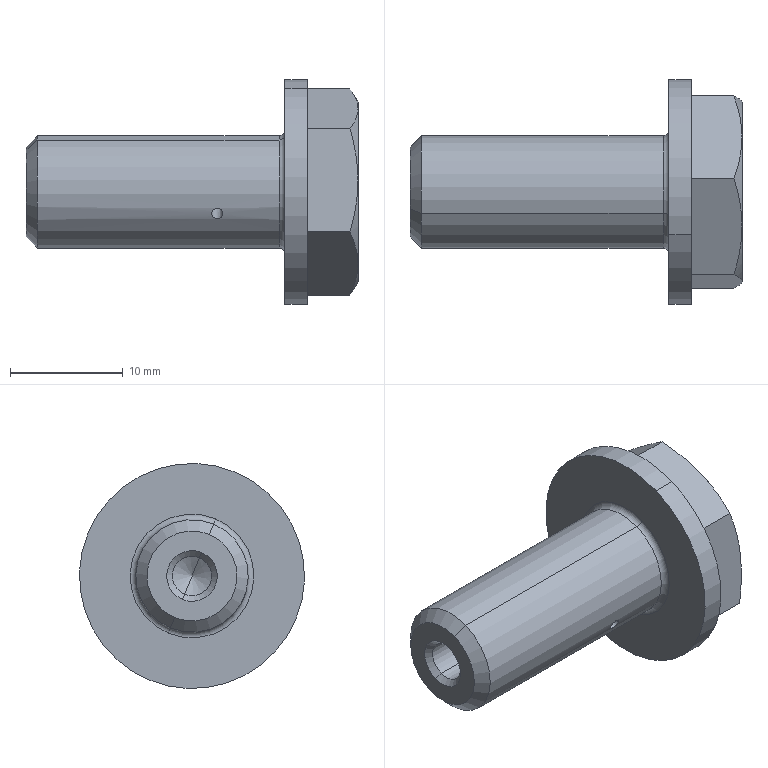Part | SolidWorks | features BaseBody 1 | 1 solid | 32 faces | box 29.5 x 20 x 20 mm | volume 3225 mm3 | cone 12 | plane 10 | cylinder 8 | torus 2 | commonest cylinder face diameters 1 x2 3.5 x2 10 x2 20 x2
STEP:
#1=CARTESIAN_POINT('',(464.9,22.643,5.081));
#2=VERTEX_POINT('',#1);
#3=CARTESIAN_POINT('',(464.9,26.857,-5.081));
#4=VERTEX_POINT('',#3);
#5=CARTESIAN_POINT('',(464.9,24.75,0.));
#6=DIRECTION('',(1.,0.,0.));
#7=DIRECTION('',(0.,0.383,-0.9237));
#8=AXIS2_PLACEMENT_3D('',#5,#6,#7);
#9=CIRCLE('',#8,5.5);
#10=EDGE_CURVE('',#2,#4,#9,.T.);
#11=ORIENTED_EDGE('',*,*,#10,.F.);
#12=CARTESIAN_POINT('',(464.4,22.835,4.619));
#13=VERTEX_POINT('',#12);
#14=CARTESIAN_POINT('',(464.4,22.643,5.081));
#15=DIRECTION('',(0.,0.9237,0.383));
#16=DIRECTION('',(0.,-0.383,0.9237));
#17=AXIS2_PLACEMENT_3D('',#14,#15,#16);
#18=CIRCLE('',#17,0.5);
#19=EDGE_CURVE('',#2,#13,#18,.T.);
#20=ORIENTED_EDGE('',*,*,#19,.T.);
#21=CARTESIAN_POINT('',(464.4,26.665,-4.619));
#22=VERTEX_POINT('',#21);
#23=CARTESIAN_POINT('',(464.4,24.75,0.));
#24=DIRECTION('',(-1.,0.,0.));
#25=DIRECTION('',(0.,0.383,-0.9237));
#26=AXIS2_PLACEMENT_3D('',#23,#24,#25);
#27=CIRCLE('',#26,5.);
#28=EDGE_CURVE('',#22,#13,#27,.T.);
#29=ORIENTED_EDGE('',*,*,#28,.F.);
#30=CARTESIAN_POINT('',(464.4,26.857,-5.081));
#31=DIRECTION('',(0.,-0.9237,-0.383));
#32=DIRECTION('',(0.,0.383,-0.9237));
#33=AXIS2_PLACEMENT_3D('',#30,#31,#32);
#34=CIRCLE('',#33,0.5);
#35=EDGE_CURVE('',#4,#22,#34,.T.);
#36=ORIENTED_EDGE('',*,*,#35,.F.);
#37=EDGE_LOOP('',(#11,#20,#29,#36));
#38=FACE_OUTER_BOUND('',#37,.T.);
#39=CARTESIAN_POINT('',(464.4,24.75,0.));
#40=DIRECTION('',(1.,0.,0.));
#41=DIRECTION('',(0.,0.383,-0.9237));
#42=AXIS2_PLACEMENT_3D('',#39,#40,#41);
#43=TOROIDAL_SURFACE('',#42,5.5,0.5);
#44=ADVANCED_FACE('',(#38),#43,.F.);
#45=CARTESIAN_POINT('',(442.4,25.42,-1.617));
#46=VERTEX_POINT('',#45);
#47=CARTESIAN_POINT('',(442.4,24.08,1.617));
#48=VERTEX_POINT('',#47);
#49=CARTESIAN_POINT('',(442.4,24.75,0.));
#50=DIRECTION('',(-1.,0.,0.));
#51=DIRECTION('',(0.,-0.383,0.9237));
#52=AXIS2_PLACEMENT_3D('',#49,#50,#51);
#53=CIRCLE('',#52,1.75);
#54=EDGE_CURVE('',#46,#48,#53,.T.);
#55=ORIENTED_EDGE('',*,*,#54,.F.);
#56=CARTESIAN_POINT('',(441.9,25.612,-2.078));
#57=VERTEX_POINT('',#56);
#58=CARTESIAN_POINT('',(442.4,25.42,-1.617));
#59=DIRECTION('',(-0.7071,0.2709,-0.6532));
#60=VECTOR('',#59,1000.);
#61=LINE('',#58,#60);
#62=EDGE_CURVE('',#46,#57,#61,.T.);
#63=ORIENTED_EDGE('',*,*,#62,.T.);
#64=CARTESIAN_POINT('',(441.9,23.888,2.078));
#65=VERTEX_POINT('',#64);
#66=CARTESIAN_POINT('',(441.9,24.75,0.));
#67=DIRECTION('',(1.,0.,0.));
#68=DIRECTION('',(0.,-0.383,0.9237));
#69=AXIS2_PLACEMENT_3D('',#66,#67,#68);
#70=CIRCLE('',#69,2.25);
#71=EDGE_CURVE('',#65,#57,#70,.T.);
#72=ORIENTED_EDGE('',*,*,#71,.F.);
#73=CARTESIAN_POINT('',(442.4,24.08,1.617));
#74=DIRECTION('',(-0.7071,-0.2709,0.6532));
#75=VECTOR('',#74,1000.);
#76=LINE('',#73,#75);
#77=EDGE_CURVE('',#48,#65,#76,.T.);
#78=ORIENTED_EDGE('',*,*,#77,.F.);
#79=EDGE_LOOP('',(#55,#63,#72,#78));
#80=FACE_OUTER_BOUND('',#79,.T.);
#81=CARTESIAN_POINT('',(442.4,24.75,0.));
#82=DIRECTION('',(-1.,0.,0.));
#83=DIRECTION('',(0.,-0.383,0.9237));
#84=AXIS2_PLACEMENT_3D('',#81,#82,#83);
#85=CONICAL_SURFACE('',#84,1.75,0.7854);
#86=ADVANCED_FACE('',(#80),#85,.F.);
#87=CARTESIAN_POINT('',(461.91,24.75,0.));
#88=VERTEX_POINT('',#87);
#89=CARTESIAN_POINT('',(460.9,24.08,1.617));
#90=VERTEX_POINT('',#89);
#91=CARTESIAN_POINT('',(460.9,24.08,1.617));
#92=DIRECTION('',(-0.5,-0.3317,0.8));
#93=VECTOR('',#92,1000.);
#94=LINE('',#91,#93);
#95=EDGE_CURVE('',#88,#90,#94,.T.);
#96=ORIENTED_EDGE('',*,*,#95,.F.);
#97=CARTESIAN_POINT('',(460.9,25.42,-1.617));
#98=VERTEX_POINT('',#97);
#99=CARTESIAN_POINT('',(460.9,25.42,-1.617));
#100=DIRECTION('',(-0.5,0.3317,-0.8));
#101=VECTOR('',#100,1000.);
#102=LINE('',#99,#101);
#103=EDGE_CURVE('',#88,#98,#102,.T.);
#104=ORIENTED_EDGE('',*,*,#103,.T.);
#105=CARTESIAN_POINT('',(460.9,24.75,0.));
#106=DIRECTION('',(-1.,0.,0.));
#107=DIRECTION('',(0.,-0.383,0.9237));
#108=AXIS2_PLACEMENT_3D('',#105,#106,#107);
#109=CIRCLE('',#108,1.75);
#110=EDGE_CURVE('',#98,#90,#109,.T.);
#111=ORIENTED_EDGE('',*,*,#110,.T.);
#112=EDGE_LOOP('',(#96,#104,#111));
#113=FACE_OUTER_BOUND('',#112,.T.);
#114=CARTESIAN_POINT('',(460.9,24.75,0.));
#115=DIRECTION('',(-1.,0.,0.));
#116=DIRECTION('',(0.,-0.383,0.9237));
#117=AXIS2_PLACEMENT_3D('',#114,#115,#116);
#118=CONICAL_SURFACE('',#117,1.75,1.047);
#119=ADVANCED_FACE('',(#113),#118,.F.);
#120=CARTESIAN_POINT('',(458.4,23.133,-0.6703));
#121=VERTEX_POINT('',#120);
#122=CARTESIAN_POINT('',(459.4,23.133,-0.6703));
#123=VERTEX_POINT('',#122);
#124=CARTESIAN_POINT('',(458.4,23.133,-0.6703));
#125=CARTESIAN_POINT('',(458.4,23.083,-0.5476));
#126=CARTESIAN_POINT('',(458.455,23.049,-0.4218));
#127=CARTESIAN_POINT('',(458.638,23.014,-0.2378));
#128=CARTESIAN_POINT('',(458.769,23.009,-0.1806));
#129=CARTESIAN_POINT('',(459.031,23.009,-0.1805));
#130=CARTESIAN_POINT('',(459.161,23.014,-0.2374));
#131=CARTESIAN_POINT('',(459.346,23.049,-0.4227));
#132=CARTESIAN_POINT('',(459.4,23.083,-0.5494));
#133=CARTESIAN_POINT('',(459.4,23.133,-0.6703));
#134=B_SPLINE_CURVE_WITH_KNOTS('',3,(#124,#125,#126,#127,#128,#129,#130,#131,#132,#133),.UNSPECIFIED.,.F.,.F.,(4,2,2,2,4),(0.,0.0003929,0.0007857,0.001179,0.001571),.UNSPECIFIED.);
#135=EDGE_CURVE('',#121,#123,#134,.T.);
#136=ORIENTED_EDGE('',*,*,#135,.F.);
#137=CARTESIAN_POINT('',(459.4,23.133,-0.6703));
#138=CARTESIAN_POINT('',(459.4,23.184,-0.7913));
#139=CARTESIAN_POINT('',(459.346,23.249,-0.9051));
#140=CARTESIAN_POINT('',(459.161,23.355,-1.061));
#141=CARTESIAN_POINT('',(459.032,23.392,-1.104));
#142=CARTESIAN_POINT('',(458.768,23.392,-1.104));
#143=CARTESIAN_POINT('',(458.638,23.355,-1.061));
#144=CARTESIAN_POINT('',(458.455,23.25,-0.9058));
#145=CARTESIAN_POINT('',(458.4,23.184,-0.7931));
#146=CARTESIAN_POINT('',(458.4,23.133,-0.6703));
#147=B_SPLINE_CURVE_WITH_KNOTS('',3,(#137,#138,#139,#140,#141,#142,#143,#144,#145,#146),.UNSPECIFIED.,.F.,.F.,(4,2,2,2,4),(0.001571,0.001964,0.002357,0.00275,0.003142),.UNSPECIFIED.);
#148=EDGE_CURVE('',#123,#121,#147,.T.);
#149=ORIENTED_EDGE('',*,*,#148,.F.);
#150=EDGE_LOOP('',(#136,#149));
#151=FACE_BOUND('',#150,.T.);
#152=ORIENTED_EDGE('',*,*,#110,.F.);
#153=CARTESIAN_POINT('',(441.9,25.42,-1.617));
#154=DIRECTION('',(-1.,0.,0.));
#155=VECTOR('',#154,1000.);
#156=LINE('',#153,#155);
#157=EDGE_CURVE('',#98,#46,#156,.T.);
#158=ORIENTED_EDGE('',*,*,#157,.T.);
#159=ORIENTED_EDGE('',*,*,#54,.T.);
#160=CARTESIAN_POINT('',(441.9,24.08,1.617));
#161=DIRECTION('',(-1.,0.,0.));
#162=VECTOR('',#161,1000.);
#163=LINE('',#160,#162);
#164=EDGE_CURVE('',#90,#48,#163,.T.);
#165=ORIENTED_EDGE('',*,*,#164,.F.);
#166=EDGE_LOOP('',(#152,#158,#159,#165));
#167=FACE_OUTER_BOUND('',#166,.T.);
#168=CARTESIAN_POINT('',(441.9,24.75,0.));
#169=DIRECTION('',(-1.,0.,0.));
#170=DIRECTION('',(0.,-0.383,0.9237));
#171=AXIS2_PLACEMENT_3D('',#168,#169,#170);
#172=CYLINDRICAL_SURFACE('',#171,1.75);
#173=ADVANCED_FACE('',(#151,#167),#172,.F.);
#174=CARTESIAN_POINT('',(466.9,20.92,9.237));
#175=VERTEX_POINT('',#174);
#176=CARTESIAN_POINT('',(466.9,28.58,-9.237));
#177=VERTEX_POINT('',#176);
#178=CARTESIAN_POINT('',(466.9,24.75,0.));
#179=DIRECTION('',(-1.,0.,0.));
#180=DIRECTION('',(0.,-0.383,0.9237));
#181=AXIS2_PLACEMENT_3D('',#178,#179,#180);
#182=CIRCLE('',#181,10.);
#183=EDGE_CURVE('',#175,#177,#182,.T.);
#184=ORIENTED_EDGE('',*,*,#183,.T.);
#185=CARTESIAN_POINT('',(464.9,28.58,-9.237));
#186=VERTEX_POINT('',#185);
#187=CARTESIAN_POINT('',(466.9,28.58,-9.237));
#188=DIRECTION('',(-1.,0.,0.));
#189=VECTOR('',#188,1000.);
#190=LINE('',#187,#189);
#191=EDGE_CURVE('',#177,#186,#190,.T.);
#192=ORIENTED_EDGE('',*,*,#191,.T.);
#193=CARTESIAN_POINT('',(464.9,20.92,9.237));
#194=VERTEX_POINT('',#193);
#195=CARTESIAN_POINT('',(464.9,24.75,0.));
#196=DIRECTION('',(-1.,0.,0.));
#197=DIRECTION('',(0.,-0.383,0.9237));
#198=AXIS2_PLACEMENT_3D('',#195,#196,#197);
#199=CIRCLE('',#198,10.);
#200=EDGE_CURVE('',#194,#186,#199,.T.);
#201=ORIENTED_EDGE('',*,*,#200,.F.);
#202=CARTESIAN_POINT('',(466.9,20.92,9.237));
#203=DIRECTION('',(-1.,0.,0.));
#204=VECTOR('',#203,1000.);
#205=LINE('',#202,#204);
#206=EDGE_CURVE('',#175,#194,#205,.T.);
#207=ORIENTED_EDGE('',*,*,#206,.F.);
#208=EDGE_LOOP('',(#184,#192,#201,#207));
#209=FACE_OUTER_BOUND('',#208,.T.);
#210=CARTESIAN_POINT('',(466.9,24.75,0.));
#211=DIRECTION('',(-1.,0.,0.));
#212=DIRECTION('',(0.,-0.383,0.9237));
#213=AXIS2_PLACEMENT_3D('',#210,#211,#212);
#214=CYLINDRICAL_SURFACE('',#213,10.);
#215=ADVANCED_FACE('',(#209),#214,.T.);
#216=CARTESIAN_POINT('',(459.4,20.131,-1.915));
#217=VERTEX_POINT('',#216);
#218=CARTESIAN_POINT('',(458.4,20.131,-1.915));
#219=VERTEX_POINT('',#218);
#220=CARTESIAN_POINT('',(459.4,20.131,-1.915));
#221=CARTESIAN_POINT('',(459.4,20.181,-2.036));
#222=CARTESIAN_POINT('',(459.346,20.237,-2.154));
#223=CARTESIAN_POINT('',(459.162,20.32,-2.32));
#224=CARTESIAN_POINT('',(459.033,20.346,-2.367));
#225=CARTESIAN_POINT('',(458.768,20.346,-2.368));
#226=CARTESIAN_POINT('',(458.639,20.32,-2.32));
#227=CARTESIAN_POINT('',(458.454,20.237,-2.155));
#228=CARTESIAN_POINT('',(458.4,20.182,-2.037));
#229=CARTESIAN_POINT('',(458.4,20.131,-1.915));
#230=B_SPLINE_CURVE_WITH_KNOTS('',3,(#220,#221,#222,#223,#224,#225,#226,#227,#228,#229),.UNSPECIFIED.,.F.,.F.,(4,2,2,2,4),(0.001564,0.001955,0.002346,0.002737,0.003128),.UNSPECIFIED.);
#231=EDGE_CURVE('',#217,#219,#230,.T.);
#232=ORIENTED_EDGE('',*,*,#231,.F.);
#233=CARTESIAN_POINT('',(459.4,16.217,-3.538));
#234=DIRECTION('',(0.,0.9237,0.383));
#235=VECTOR('',#234,1000.);
#236=LINE('',#233,#235);
#237=EDGE_CURVE('',#217,#123,#236,.T.);
#238=ORIENTED_EDGE('',*,*,#237,.T.);
#239=ORIENTED_EDGE('',*,*,#148,.T.);
#240=CARTESIAN_POINT('',(458.4,16.217,-3.538));
#241=DIRECTION('',(0.,0.9237,0.383));
#242=VECTOR('',#241,1000.);
#243=LINE('',#240,#242);
#244=EDGE_CURVE('',#219,#121,#243,.T.);
#245=ORIENTED_EDGE('',*,*,#244,.F.);
#246=EDGE_LOOP('',(#232,#238,#239,#245));
#247=FACE_OUTER_BOUND('',#246,.T.);
#248=CARTESIAN_POINT('',(458.9,16.217,-3.538));
#249=DIRECTION('',(0.,0.9237,0.383));
#250=DIRECTION('',(-1.,0.,0.));
#251=AXIS2_PLACEMENT_3D('',#248,#249,#250);
#252=CYLINDRICAL_SURFACE('',#251,0.5);
#253=ADVANCED_FACE('',(#247),#252,.F.);
#254=CARTESIAN_POINT('',(441.9,23.218,3.695));
#255=VERTEX_POINT('',#254);
#256=CARTESIAN_POINT('',(441.9,26.282,-3.695));
#257=VERTEX_POINT('',#256);
#258=CARTESIAN_POINT('',(441.9,24.75,0.));
#259=DIRECTION('',(-1.,0.,0.));
#260=DIRECTION('',(0.,-0.383,0.9237));
#261=AXIS2_PLACEMENT_3D('',#258,#259,#260);
#262=CIRCLE('',#261,4.);
#263=EDGE_CURVE('',#255,#257,#262,.T.);
#264=ORIENTED_EDGE('',*,*,#263,.F.);
#265=CARTESIAN_POINT('',(442.9,22.835,4.619));
#266=VERTEX_POINT('',#265);
#267=CARTESIAN_POINT('',(441.9,23.218,3.695));
#268=DIRECTION('',(0.7071,-0.2709,0.6532));
#269=VECTOR('',#268,1000.);
#270=LINE('',#267,#269);
#271=EDGE_CURVE('',#255,#266,#270,.T.);
#272=ORIENTED_EDGE('',*,*,#271,.T.);
#273=CARTESIAN_POINT('',(442.9,26.665,-4.619));
#274=VERTEX_POINT('',#273);
#275=CARTESIAN_POINT('',(442.9,24.75,0.));
#276=DIRECTION('',(1.,0.,0.));
#277=DIRECTION('',(0.,-0.383,0.9237));
#278=AXIS2_PLACEMENT_3D('',#275,#276,#277);
#279=CIRCLE('',#278,5.);
#280=EDGE_CURVE('',#274,#266,#279,.T.);
#281=ORIENTED_EDGE('',*,*,#280,.F.);
#282=CARTESIAN_POINT('',(441.9,26.282,-3.695));
#283=DIRECTION('',(0.7071,0.2709,-0.6532));
#284=VECTOR('',#283,1000.);
#285=LINE('',#282,#284);
#286=EDGE_CURVE('',#257,#274,#285,.T.);
#287=ORIENTED_EDGE('',*,*,#286,.F.);
#288=EDGE_LOOP('',(#264,#272,#281,#287));
#289=FACE_OUTER_BOUND('',#288,.T.);
#290=CARTESIAN_POINT('',(441.9,24.75,0.));
#291=DIRECTION('',(1.,0.,0.));
#292=DIRECTION('',(0.,0.383,-0.9237));
#293=AXIS2_PLACEMENT_3D('',#290,#291,#292);
#294=CONICAL_SURFACE('',#293,4.,0.7854);
#295=ADVANCED_FACE('',(#289),#294,.T.);
#296=ORIENTED_EDGE('',*,*,#280,.T.);
#297=CARTESIAN_POINT('',(441.9,22.835,4.619));
#298=DIRECTION('',(1.,0.,0.));
#299=VECTOR('',#298,1000.);
#300=LINE('',#297,#299);
#301=EDGE_CURVE('',#266,#13,#300,.T.);
#302=ORIENTED_EDGE('',*,*,#301,.T.);
#303=CARTESIAN_POINT('',(464.4,24.75,0.));
#304=DIRECTION('',(-1.,0.,0.));
#305=DIRECTION('',(0.,0.383,-0.9237));
#306=AXIS2_PLACEMENT_3D('',#303,#304,#305);
#307=CIRCLE('',#306,5.);
#308=EDGE_CURVE('',#13,#22,#307,.T.);
#309=ORIENTED_EDGE('',*,*,#308,.T.);
#310=CARTESIAN_POINT('',(441.9,26.665,-4.619));
#311=DIRECTION('',(1.,0.,0.));
#312=VECTOR('',#311,1000.);
#313=LINE('',#310,#312);
#314=EDGE_CURVE('',#274,#22,#313,.T.);
#315=ORIENTED_EDGE('',*,*,#314,.F.);
#316=EDGE_LOOP('',(#296,#302,#309,#315));
#317=FACE_OUTER_BOUND('',#316,.T.);
#318=CARTESIAN_POINT('',(441.9,24.75,0.));
#319=DIRECTION('',(1.,0.,0.));
#320=DIRECTION('',(0.,0.383,-0.9237));
#321=AXIS2_PLACEMENT_3D('',#318,#319,#320);
#322=CYLINDRICAL_SURFACE('',#321,5.);
#323=ADVANCED_FACE('',(#317),#322,.T.);
#324=CARTESIAN_POINT('',(464.9,24.75,0.));
#325=DIRECTION('',(1.,0.,0.));
#326=DIRECTION('',(0.,0.383,-0.9237));
#327=AXIS2_PLACEMENT_3D('',#324,#325,#326);
#328=CIRCLE('',#327,5.5);
#329=EDGE_CURVE('',#4,#2,#328,.T.);
#330=ORIENTED_EDGE('',*,*,#329,.T.);
#331=ORIENTED_EDGE('',*,*,#10,.T.);
#332=EDGE_LOOP('',(#330,#331));
#333=FACE_BOUND('',#332,.T.);
#334=ORIENTED_EDGE('',*,*,#200,.T.);
#335=CARTESIAN_POINT('',(464.9,24.75,0.));
#336=DIRECTION('',(-1.,0.,0.));
#337=DIRECTION('',(0.,-0.383,0.9237));
#338=AXIS2_PLACEMENT_3D('',#335,#336,#337);
#339=CIRCLE('',#338,10.);
#340=EDGE_CURVE('',#186,#194,#339,.T.);
#341=ORIENTED_EDGE('',*,*,#340,.T.);
#342=EDGE_LOOP('',(#334,#341));
#343=FACE_OUTER_BOUND('',#342,.T.);
#344=CARTESIAN_POINT('',(464.9,30.879,-14.78));
#345=DIRECTION('',(1.,0.,0.));
#346=DIRECTION('',(0.,0.383,-0.9237));
#347=AXIS2_PLACEMENT_3D('',#344,#345,#346);
#348=PLANE('',#347);
#349=ADVANCED_FACE('',(#333,#343),#348,.F.);
#350=ORIENTED_EDGE('',*,*,#301,.F.);
#351=CARTESIAN_POINT('',(442.9,24.75,0.));
#352=DIRECTION('',(1.,0.,0.));
#353=DIRECTION('',(0.,-0.383,0.9237));
#354=AXIS2_PLACEMENT_3D('',#351,#352,#353);
#355=CIRCLE('',#354,5.);
#356=EDGE_CURVE('',#266,#274,#355,.T.);
#357=ORIENTED_EDGE('',*,*,#356,.T.);
#358=ORIENTED_EDGE('',*,*,#314,.T.);
#359=ORIENTED_EDGE('',*,*,#28,.T.);
#360=EDGE_LOOP('',(#350,#357,#358,#359));
#361=FACE_OUTER_BOUND('',#360,.T.);
#362=CARTESIAN_POINT('',(458.4,20.131,-1.915));
#363=CARTESIAN_POINT('',(458.4,20.081,-1.793));
#364=CARTESIAN_POINT('',(458.454,20.037,-1.671));
#365=CARTESIAN_POINT('',(458.639,19.978,-1.496));
#366=CARTESIAN_POINT('',(458.769,19.963,-1.444));
#367=CARTESIAN_POINT('',(459.03,19.963,-1.444));
#368=CARTESIAN_POINT('',(459.16,19.978,-1.495));
#369=CARTESIAN_POINT('',(459.347,20.037,-1.673));
#370=CARTESIAN_POINT('',(459.4,20.081,-1.795));
#371=CARTESIAN_POINT('',(459.4,20.131,-1.915));
#372=B_SPLINE_CURVE_WITH_KNOTS('',3,(#362,#363,#364,#365,#366,#367,#368,#369,#370,#371),.UNSPECIFIED.,.F.,.F.,(4,2,2,2,4),(0.,0.0003911,0.0007821,0.001173,0.001564),.UNSPECIFIED.);
#373=EDGE_CURVE('',#219,#217,#372,.T.);
#374=ORIENTED_EDGE('',*,*,#373,.T.);
#375=ORIENTED_EDGE('',*,*,#231,.T.);
#376=EDGE_LOOP('',(#374,#375));
#377=FACE_BOUND('',#376,.T.);
#378=CARTESIAN_POINT('',(441.9,24.75,0.));
#379=DIRECTION('',(1.,0.,0.));
#380=DIRECTION('',(0.,0.383,-0.9237));
#381=AXIS2_PLACEMENT_3D('',#378,#379,#380);
#382=CYLINDRICAL_SURFACE('',#381,5.);
#383=ADVANCED_FACE('',(#361,#377),#382,.T.);
#384=ORIENTED_EDGE('',*,*,#71,.T.);
#385=CARTESIAN_POINT('',(441.9,24.75,0.));
#386=DIRECTION('',(1.,0.,0.));
#387=DIRECTION('',(0.,-0.383,0.9237));
#388=AXIS2_PLACEMENT_3D('',#385,#386,#387);
#389=CIRCLE('',#388,2.25);
#390=EDGE_CURVE('',#57,#65,#389,.T.);
#391=ORIENTED_EDGE('',*,*,#390,.T.);
#392=EDGE_LOOP('',(#384,#391));
#393=FACE_BOUND('',#392,.T.);
#394=CARTESIAN_POINT('',(441.9,24.75,0.));
#395=DIRECTION('',(-1.,0.,0.));
#396=DIRECTION('',(0.,-0.383,0.9237));
#397=AXIS2_PLACEMENT_3D('',#394,#395,#396);
#398=CIRCLE('',#397,4.);
#399=EDGE_CURVE('',#257,#255,#398,.T.);
#400=ORIENTED_EDGE('',*,*,#399,.T.);
#401=ORIENTED_EDGE('',*,*,#263,.T.);
#402=EDGE_LOOP('',(#400,#401));
#403=FACE_OUTER_BOUND('',#402,.T.);
#404=CARTESIAN_POINT('',(441.9,24.75,0.));
#405=DIRECTION('',(-1.,0.,0.));
#406=DIRECTION('',(0.,-0.383,0.9237));
#407=AXIS2_PLACEMENT_3D('',#404,#405,#406);
#408=PLANE('',#407);
#409=ADVANCED_FACE('',(#393,#403),#408,.T.);
#410=ORIENTED_EDGE('',*,*,#271,.F.);
#411=ORIENTED_EDGE('',*,*,#399,.F.);
#412=ORIENTED_EDGE('',*,*,#286,.T.);
#413=ORIENTED_EDGE('',*,*,#356,.F.);
#414=EDGE_LOOP('',(#410,#411,#412,#413));
#415=FACE_OUTER_BOUND('',#414,.T.);
#416=CARTESIAN_POINT('',(441.9,24.75,0.));
#417=DIRECTION('',(1.,0.,0.));
#418=DIRECTION('',(0.,0.383,-0.9237));
#419=AXIS2_PLACEMENT_3D('',#416,#417,#418);
#420=CONICAL_SURFACE('',#419,4.,0.7854);
#421=ADVANCED_FACE('',(#415),#420,.T.);
#422=ORIENTED_EDGE('',*,*,#237,.F.);
#423=ORIENTED_EDGE('',*,*,#373,.F.);
#424=ORIENTED_EDGE('',*,*,#244,.T.);
#425=ORIENTED_EDGE('',*,*,#135,.T.);
#426=EDGE_LOOP('',(#422,#423,#424,#425));
#427=FACE_OUTER_BOUND('',#426,.T.);
#428=CARTESIAN_POINT('',(458.9,16.217,-3.538));
#429=DIRECTION('',(0.,0.9237,0.383));
#430=DIRECTION('',(-1.,0.,0.));
#431=AXIS2_PLACEMENT_3D('',#428,#429,#430);
#432=CYLINDRICAL_SURFACE('',#431,0.5);
#433=ADVANCED_FACE('',(#427),#432,.F.);
#434=ORIENTED_EDGE('',*,*,#183,.F.);
#435=CARTESIAN_POINT('',(466.9,24.75,0.));
#436=DIRECTION('',(-1.,0.,0.));
#437=DIRECTION('',(0.,-0.383,0.9237));
#438=AXIS2_PLACEMENT_3D('',#435,#436,#437);
#439=CIRCLE('',#438,10.);
#440=EDGE_CURVE('',#177,#175,#439,.T.);
#441=ORIENTED_EDGE('',*,*,#440,.F.);
#442=EDGE_LOOP('',(#434,#441));
#443=FACE_OUTER_BOUND('',#442,.T.);
#444=CARTESIAN_POINT('',(466.9,25.952,9.159));
#445=VERTEX_POINT('',#444);
#446=CARTESIAN_POINT('',(466.9,33.283,3.538));
#447=VERTEX_POINT('',#446);
#448=CARTESIAN_POINT('',(466.9,33.283,3.538));
#449=DIRECTION('',(0.,0.7936,-0.6084));
#450=VECTOR('',#449,1000.);
#451=LINE('',#448,#450);
#452=EDGE_CURVE('',#445,#447,#451,.T.);
#453=ORIENTED_EDGE('',*,*,#452,.T.);
#454=CARTESIAN_POINT('',(466.9,32.081,-5.621));
#455=VERTEX_POINT('',#454);
#456=CARTESIAN_POINT('',(466.9,33.283,3.538));
#457=DIRECTION('',(0.,-0.1301,-0.9915));
#458=VECTOR('',#457,1000.);
#459=LINE('',#456,#458);
#460=EDGE_CURVE('',#447,#455,#459,.T.);
#461=ORIENTED_EDGE('',*,*,#460,.T.);
#462=CARTESIAN_POINT('',(466.9,23.548,-9.159));
#463=VERTEX_POINT('',#462);
#464=CARTESIAN_POINT('',(466.9,23.548,-9.159));
#465=DIRECTION('',(0.,-0.9237,-0.383));
#466=VECTOR('',#465,1000.);
#467=LINE('',#464,#466);
#468=EDGE_CURVE('',#455,#463,#467,.T.);
#469=ORIENTED_EDGE('',*,*,#468,.T.);
#470=CARTESIAN_POINT('',(466.9,16.217,-3.538));
#471=VERTEX_POINT('',#470);
#472=CARTESIAN_POINT('',(466.9,16.217,-3.538));
#473=DIRECTION('',(0.,-0.7936,0.6084));
#474=VECTOR('',#473,1000.);
#475=LINE('',#472,#474);
#476=EDGE_CURVE('',#463,#471,#475,.T.);
#477=ORIENTED_EDGE('',*,*,#476,.T.);
#478=CARTESIAN_POINT('',(466.9,17.419,5.621));
#479=VERTEX_POINT('',#478);
#480=CARTESIAN_POINT('',(466.9,16.217,-3.538));
#481=DIRECTION('',(0.,0.1301,0.9915));
#482=VECTOR('',#481,1000.);
#483=LINE('',#480,#482);
#484=EDGE_CURVE('',#471,#479,#483,.T.);
#485=ORIENTED_EDGE('',*,*,#484,.T.);
#486=CARTESIAN_POINT('',(466.9,25.952,9.159));
#487=DIRECTION('',(0.,0.9237,0.383));
#488=VECTOR('',#487,1000.);
#489=LINE('',#486,#488);
#490=EDGE_CURVE('',#479,#445,#489,.T.);
#491=ORIENTED_EDGE('',*,*,#490,.T.);
#492=EDGE_LOOP('',(#453,#461,#469,#477,#485,#491));
#493=FACE_BOUND('',#492,.T.);
#494=CARTESIAN_POINT('',(466.9,24.75,0.));
#495=DIRECTION('',(-1.,0.,0.));
#496=DIRECTION('',(0.,-0.383,0.9237));
#497=AXIS2_PLACEMENT_3D('',#494,#495,#496);
#498=PLANE('',#497);
#499=ADVANCED_FACE('',(#443,#493),#498,.F.);
#500=ORIENTED_EDGE('',*,*,#191,.F.);
#501=ORIENTED_EDGE('',*,*,#440,.T.);
#502=ORIENTED_EDGE('',*,*,#206,.T.);
#503=ORIENTED_EDGE('',*,*,#340,.F.);
#504=EDGE_LOOP('',(#500,#501,#502,#503));
#505=FACE_OUTER_BOUND('',#504,.T.);
#506=CARTESIAN_POINT('',(466.9,24.75,0.));
#507=DIRECTION('',(-1.,0.,0.));
#508=DIRECTION('',(0.,-0.383,0.9237));
#509=AXIS2_PLACEMENT_3D('',#506,#507,#508);
#510=CYLINDRICAL_SURFACE('',#509,10.);
#511=ADVANCED_FACE('',(#505),#510,.T.);
#512=CARTESIAN_POINT('',(471.4,27.814,-7.39));
#513=VERTEX_POINT('',#512);
#514=CARTESIAN_POINT('',(471.4,32.682,-1.041));
#515=VERTEX_POINT('',#514);
#516=CARTESIAN_POINT('',(471.4,24.75,0.));
#517=DIRECTION('',(1.,0.,0.));
#518=DIRECTION('',(0.,0.383,-0.9237));
#519=AXIS2_PLACEMENT_3D('',#516,#517,#518);
#520=CIRCLE('',#519,8.);
#521=EDGE_CURVE('',#513,#515,#520,.T.);
#522=ORIENTED_EDGE('',*,*,#521,.T.);
#523=CARTESIAN_POINT('',(471.4,29.618,6.349));
#524=VERTEX_POINT('',#523);
#525=CARTESIAN_POINT('',(471.4,24.75,0.));
#526=DIRECTION('',(1.,0.,0.));
#527=DIRECTION('',(0.,0.383,-0.9237));
#528=AXIS2_PLACEMENT_3D('',#525,#526,#527);
#529=CIRCLE('',#528,8.);
#530=EDGE_CURVE('',#515,#524,#529,.T.);
#531=ORIENTED_EDGE('',*,*,#530,.T.);
#532=CARTESIAN_POINT('',(471.4,21.686,7.39));
#533=VERTEX_POINT('',#532);
#534=CARTESIAN_POINT('',(471.4,24.75,0.));
#535=DIRECTION('',(1.,0.,0.));
#536=DIRECTION('',(0.,0.383,-0.9237));
#537=AXIS2_PLACEMENT_3D('',#534,#535,#536);
#538=CIRCLE('',#537,8.);
#539=EDGE_CURVE('',#524,#533,#538,.T.);
#540=ORIENTED_EDGE('',*,*,#539,.T.);
#541=CARTESIAN_POINT('',(471.4,16.818,1.041));
#542=VERTEX_POINT('',#541);
#543=CARTESIAN_POINT('',(471.4,24.75,0.));
#544=DIRECTION('',(1.,0.,0.));
#545=DIRECTION('',(0.,0.383,-0.9237));
#546=AXIS2_PLACEMENT_3D('',#543,#544,#545);
#547=CIRCLE('',#546,8.);
#548=EDGE_CURVE('',#533,#542,#547,.T.);
#549=ORIENTED_EDGE('',*,*,#548,.T.);
#550=CARTESIAN_POINT('',(471.4,19.882,-6.349));
#551=VERTEX_POINT('',#550);
#552=CARTESIAN_POINT('',(471.4,24.75,0.));
#553=DIRECTION('',(1.,0.,0.));
#554=DIRECTION('',(0.,0.383,-0.9237));
#555=AXIS2_PLACEMENT_3D('',#552,#553,#554);
#556=CIRCLE('',#555,8.);
#557=EDGE_CURVE('',#542,#551,#556,.T.);
#558=ORIENTED_EDGE('',*,*,#557,.T.);
#559=CARTESIAN_POINT('',(471.4,24.75,0.));
#560=DIRECTION('',(1.,0.,0.));
#561=DIRECTION('',(0.,0.383,-0.9237));
#562=AXIS2_PLACEMENT_3D('',#559,#560,#561);
#563=CIRCLE('',#562,8.);
#564=EDGE_CURVE('',#551,#513,#563,.T.);
#565=ORIENTED_EDGE('',*,*,#564,.T.);
#566=EDGE_LOOP('',(#522,#531,#540,#549,#558,#565));
#567=FACE_OUTER_BOUND('',#566,.T.);
#568=CARTESIAN_POINT('',(471.4,30.879,-14.78));
#569=DIRECTION('',(1.,0.,0.));
#570=DIRECTION('',(0.,0.383,-0.9237));
#571=AXIS2_PLACEMENT_3D('',#568,#569,#570);
#572=PLANE('',#571);
#573=ADVANCED_FACE('',(#567),#572,.T.);
#574=CARTESIAN_POINT('',(470.685,32.081,-5.621));
#575=VERTEX_POINT('',#574);
#576=CARTESIAN_POINT('',(471.4,32.682,-1.041));
#577=CARTESIAN_POINT('',(471.4,32.631,-1.43));
#578=CARTESIAN_POINT('',(471.383,32.58,-1.82));
#579=CARTESIAN_POINT('',(471.318,32.478,-2.592));
#580=CARTESIAN_POINT('',(471.269,32.428,-2.976));
#581=CARTESIAN_POINT('',(471.083,32.278,-4.12));
#582=CARTESIAN_POINT('',(470.903,32.179,-4.873));
#583=CARTESIAN_POINT('',(470.685,32.081,-5.621));
#584=B_SPLINE_CURVE_WITH_KNOTS('',3,(#576,#577,#578,#579,#580,#581,#582,#583),.UNSPECIFIED.,.F.,.F.,(4,2,2,4),(0.004674,0.005838,0.007002,0.00933),.UNSPECIFIED.);
#585=EDGE_CURVE('',#515,#575,#584,.T.);
#586=ORIENTED_EDGE('',*,*,#585,.F.);
#587=ORIENTED_EDGE('',*,*,#521,.F.);
#588=CARTESIAN_POINT('',(470.685,32.081,-5.621));
#589=CARTESIAN_POINT('',(470.901,31.391,-5.907));
#590=CARTESIAN_POINT('',(471.081,30.692,-6.197));
#591=CARTESIAN_POINT('',(471.268,29.624,-6.639));
#592=CARTESIAN_POINT('',(471.317,29.265,-6.788));
#593=CARTESIAN_POINT('',(471.383,28.54,-7.089));
#594=CARTESIAN_POINT('',(471.4,28.176,-7.24));
#595=CARTESIAN_POINT('',(471.4,27.814,-7.39));
#596=B_SPLINE_CURVE_WITH_KNOTS('',3,(#588,#589,#590,#591,#592,#593,#594,#595),.UNSPECIFIED.,.F.,.F.,(4,2,2,4),(0.02476,0.02709,0.02826,0.02943),.UNSPECIFIED.);
#597=EDGE_CURVE('',#575,#513,#596,.T.);
#598=ORIENTED_EDGE('',*,*,#597,.F.);
#599=EDGE_LOOP('',(#586,#587,#598));
#600=FACE_OUTER_BOUND('',#599,.T.);
#601=CARTESIAN_POINT('',(471.4,24.75,0.));
#602=DIRECTION('',(-1.,0.,0.));
#603=DIRECTION('',(0.,0.383,-0.9237));
#604=AXIS2_PLACEMENT_3D('',#601,#602,#603);
#605=CONICAL_SURFACE('',#604,8.,1.047);
#606=ADVANCED_FACE('',(#600),#605,.T.);
#607=CARTESIAN_POINT('',(470.685,23.548,-9.159));
#608=VERTEX_POINT('',#607);
#609=CARTESIAN_POINT('',(471.4,27.814,-7.39));
#610=CARTESIAN_POINT('',(471.4,27.092,-7.689));
#611=CARTESIAN_POINT('',(471.333,26.376,-7.986));
#612=CARTESIAN_POINT('',(471.084,24.953,-8.576));
#613=CARTESIAN_POINT('',(470.903,24.243,-8.871));
#614=CARTESIAN_POINT('',(470.685,23.548,-9.159));
#615=B_SPLINE_CURVE_WITH_KNOTS('',3,(#609,#610,#611,#612,#613,#614),.UNSPECIFIED.,.F.,.F.,(4,2,4),(0.02943,0.03177,0.03411),.UNSPECIFIED.);
#616=EDGE_CURVE('',#513,#608,#615,.T.);
#617=ORIENTED_EDGE('',*,*,#616,.F.);
#618=ORIENTED_EDGE('',*,*,#564,.F.);
#619=CARTESIAN_POINT('',(470.685,23.548,-9.159));
#620=CARTESIAN_POINT('',(470.904,22.948,-8.699));
#621=CARTESIAN_POINT('',(471.083,22.344,-8.236));
#622=CARTESIAN_POINT('',(471.332,21.124,-7.3));
#623=CARTESIAN_POINT('',(471.4,20.507,-6.828));
#624=CARTESIAN_POINT('',(471.4,19.882,-6.349));
#625=B_SPLINE_CURVE_WITH_KNOTS('',3,(#619,#620,#621,#622,#623,#624),.UNSPECIFIED.,.F.,.F.,(4,2,4),(0.000000238,0.002337,0.004674),.UNSPECIFIED.);
#626=EDGE_CURVE('',#608,#551,#625,.T.);
#627=ORIENTED_EDGE('',*,*,#626,.F.);
#628=EDGE_LOOP('',(#617,#618,#627));
#629=FACE_OUTER_BOUND('',#628,.T.);
#630=CARTESIAN_POINT('',(471.4,24.75,0.));
#631=DIRECTION('',(-1.,0.,0.));
#632=DIRECTION('',(0.,0.383,-0.9237));
#633=AXIS2_PLACEMENT_3D('',#630,#631,#632);
#634=CONICAL_SURFACE('',#633,8.,1.047);
#635=ADVANCED_FACE('',(#629),#634,.T.);
#636=CARTESIAN_POINT('',(470.685,16.217,-3.538));
#637=VERTEX_POINT('',#636);
#638=CARTESIAN_POINT('',(471.4,19.882,-6.349));
#639=CARTESIAN_POINT('',(471.4,19.571,-6.11));
#640=CARTESIAN_POINT('',(471.383,19.259,-5.871));
#641=CARTESIAN_POINT('',(471.318,18.641,-5.397));
#642=CARTESIAN_POINT('',(471.269,18.334,-5.161));
#643=CARTESIAN_POINT('',(471.083,17.418,-4.459));
#644=CARTESIAN_POINT('',(470.903,16.815,-3.997));
#645=CARTESIAN_POINT('',(470.685,16.217,-3.538));
#646=B_SPLINE_CURVE_WITH_KNOTS('',3,(#638,#639,#640,#641,#642,#643,#644,#645),.UNSPECIFIED.,.F.,.F.,(4,2,2,4),(0.004674,0.005838,0.007002,0.00933),.UNSPECIFIED.);
#647=EDGE_CURVE('',#551,#637,#646,.T.);
#648=ORIENTED_EDGE('',*,*,#647,.F.);
#649=ORIENTED_EDGE('',*,*,#557,.F.);
#650=CARTESIAN_POINT('',(470.685,16.217,-3.538));
#651=CARTESIAN_POINT('',(470.904,16.315,-2.789));
#652=CARTESIAN_POINT('',(471.083,16.414,-2.035));
#653=CARTESIAN_POINT('',(471.332,16.614,-0.5097));
#654=CARTESIAN_POINT('',(471.4,16.716,0.2609));
#655=CARTESIAN_POINT('',(471.4,16.818,1.041));
#656=B_SPLINE_CURVE_WITH_KNOTS('',3,(#650,#651,#652,#653,#654,#655),.UNSPECIFIED.,.F.,.F.,(4,2,4),(0.000000238,0.002337,0.004674),.UNSPECIFIED.);
#657=EDGE_CURVE('',#637,#542,#656,.T.);
#658=ORIENTED_EDGE('',*,*,#657,.F.);
#659=EDGE_LOOP('',(#648,#649,#658));
#660=FACE_OUTER_BOUND('',#659,.T.);
#661=CARTESIAN_POINT('',(471.4,24.75,0.));
#662=DIRECTION('',(-1.,0.,0.));
#663=DIRECTION('',(0.,0.383,-0.9237));
#664=AXIS2_PLACEMENT_3D('',#661,#662,#663);
#665=CONICAL_SURFACE('',#664,8.,1.047);
#666=ADVANCED_FACE('',(#660),#665,.T.);
#667=CARTESIAN_POINT('',(470.685,17.419,5.621));
#668=VERTEX_POINT('',#667);
#669=CARTESIAN_POINT('',(471.4,16.818,1.041));
#670=CARTESIAN_POINT('',(471.4,16.869,1.43));
#671=CARTESIAN_POINT('',(471.383,16.92,1.82));
#672=CARTESIAN_POINT('',(471.318,17.022,2.592));
#673=CARTESIAN_POINT('',(471.269,17.072,2.976));
#674=CARTESIAN_POINT('',(471.083,17.222,4.12));
#675=CARTESIAN_POINT('',(470.903,17.321,4.873));
#676=CARTESIAN_POINT('',(470.685,17.419,5.621));
#677=B_SPLINE_CURVE_WITH_KNOTS('',3,(#669,#670,#671,#672,#673,#674,#675,#676),.UNSPECIFIED.,.F.,.F.,(4,2,2,4),(0.004674,0.005838,0.007002,0.00933),.UNSPECIFIED.);
#678=EDGE_CURVE('',#542,#668,#677,.T.);
#679=ORIENTED_EDGE('',*,*,#678,.F.);
#680=ORIENTED_EDGE('',*,*,#548,.F.);
#681=CARTESIAN_POINT('',(470.685,17.419,5.621));
#682=CARTESIAN_POINT('',(470.903,18.114,5.909));
#683=CARTESIAN_POINT('',(471.084,18.824,6.203));
#684=CARTESIAN_POINT('',(471.333,20.247,6.793));
#685=CARTESIAN_POINT('',(471.4,20.964,7.09));
#686=CARTESIAN_POINT('',(471.4,21.686,7.39));
#687=B_SPLINE_CURVE_WITH_KNOTS('',3,(#681,#682,#683,#684,#685,#686),.UNSPECIFIED.,.F.,.F.,(4,2,4),(0.008635,0.01097,0.01331),.UNSPECIFIED.);
#688=EDGE_CURVE('',#668,#533,#687,.T.);
#689=ORIENTED_EDGE('',*,*,#688,.F.);
#690=EDGE_LOOP('',(#679,#680,#689));
#691=FACE_OUTER_BOUND('',#690,.T.);
#692=CARTESIAN_POINT('',(471.4,24.75,0.));
#693=DIRECTION('',(-1.,0.,0.));
#694=DIRECTION('',(0.,0.383,-0.9237));
#695=AXIS2_PLACEMENT_3D('',#692,#693,#694);
#696=CONICAL_SURFACE('',#695,8.,1.047);
#697=ADVANCED_FACE('',(#691),#696,.T.);
#698=CARTESIAN_POINT('',(470.685,33.283,3.538));
#699=VERTEX_POINT('',#698);
#700=CARTESIAN_POINT('',(470.685,33.283,3.538));
#701=CARTESIAN_POINT('',(470.904,33.185,2.789));
#702=CARTESIAN_POINT('',(471.083,33.086,2.035));
#703=CARTESIAN_POINT('',(471.332,32.886,0.5097));
#704=CARTESIAN_POINT('',(471.4,32.784,-0.2609));
#705=CARTESIAN_POINT('',(471.4,32.682,-1.041));
#706=B_SPLINE_CURVE_WITH_KNOTS('',3,(#700,#701,#702,#703,#704,#705),.UNSPECIFIED.,.F.,.F.,(4,2,4),(0.000000238,0.002337,0.004674),.UNSPECIFIED.);
#707=EDGE_CURVE('',#699,#515,#706,.T.);
#708=ORIENTED_EDGE('',*,*,#707,.F.);
#709=CARTESIAN_POINT('',(471.4,29.618,6.349));
#710=CARTESIAN_POINT('',(471.4,29.929,6.11));
#711=CARTESIAN_POINT('',(471.383,30.241,5.871));
#712=CARTESIAN_POINT('',(471.318,30.859,5.397));
#713=CARTESIAN_POINT('',(471.269,31.166,5.161));
#714=CARTESIAN_POINT('',(471.083,32.082,4.459));
#715=CARTESIAN_POINT('',(470.903,32.685,3.997));
#716=CARTESIAN_POINT('',(470.685,33.283,3.538));
#717=B_SPLINE_CURVE_WITH_KNOTS('',3,(#709,#710,#711,#712,#713,#714,#715,#716),.UNSPECIFIED.,.F.,.F.,(4,2,2,4),(0.004674,0.005838,0.007002,0.00933),.UNSPECIFIED.);
#718=EDGE_CURVE('',#524,#699,#717,.T.);
#719=ORIENTED_EDGE('',*,*,#718,.F.);
#720=ORIENTED_EDGE('',*,*,#530,.F.);
#721=EDGE_LOOP('',(#708,#719,#720));
#722=FACE_OUTER_BOUND('',#721,.T.);
#723=CARTESIAN_POINT('',(471.4,24.75,0.));
#724=DIRECTION('',(-1.,0.,0.));
#725=DIRECTION('',(0.,0.383,-0.9237));
#726=AXIS2_PLACEMENT_3D('',#723,#724,#725);
#727=CONICAL_SURFACE('',#726,8.,1.047);
#728=ADVANCED_FACE('',(#722),#727,.T.);
#729=CARTESIAN_POINT('',(470.685,25.952,9.159));
#730=VERTEX_POINT('',#729);
#731=CARTESIAN_POINT('',(471.4,21.686,7.39));
#732=CARTESIAN_POINT('',(471.4,22.047,7.54));
#733=CARTESIAN_POINT('',(471.383,22.411,7.691));
#734=CARTESIAN_POINT('',(471.317,23.137,7.991));
#735=CARTESIAN_POINT('',(471.268,23.496,8.14));
#736=CARTESIAN_POINT('',(471.081,24.563,8.583));
#737=CARTESIAN_POINT('',(470.901,25.262,8.873));
#738=CARTESIAN_POINT('',(470.685,25.952,9.159));
#739=B_SPLINE_CURVE_WITH_KNOTS('',3,(#731,#732,#733,#734,#735,#736,#737,#738),.UNSPECIFIED.,.F.,.F.,(4,2,2,4),(0.01331,0.01448,0.01565,0.01799),.UNSPECIFIED.);
#740=EDGE_CURVE('',#533,#730,#739,.T.);
#741=ORIENTED_EDGE('',*,*,#740,.F.);
#742=ORIENTED_EDGE('',*,*,#539,.F.);
#743=CARTESIAN_POINT('',(470.685,25.952,9.159));
#744=CARTESIAN_POINT('',(470.904,26.552,8.699));
#745=CARTESIAN_POINT('',(471.083,27.156,8.236));
#746=CARTESIAN_POINT('',(471.332,28.376,7.3));
#747=CARTESIAN_POINT('',(471.4,28.993,6.828));
#748=CARTESIAN_POINT('',(471.4,29.618,6.349));
#749=B_SPLINE_CURVE_WITH_KNOTS('',3,(#743,#744,#745,#746,#747,#748),.UNSPECIFIED.,.F.,.F.,(4,2,4),(0.000000238,0.002337,0.004674),.UNSPECIFIED.);
#750=EDGE_CURVE('',#730,#524,#749,.T.);
#751=ORIENTED_EDGE('',*,*,#750,.F.);
#752=EDGE_LOOP('',(#741,#742,#751));
#753=FACE_OUTER_BOUND('',#752,.T.);
#754=CARTESIAN_POINT('',(471.4,24.75,0.));
#755=DIRECTION('',(-1.,0.,0.));
#756=DIRECTION('',(0.,0.383,-0.9237));
#757=AXIS2_PLACEMENT_3D('',#754,#755,#756);
#758=CONICAL_SURFACE('',#757,8.,1.047);
#759=ADVANCED_FACE('',(#753),#758,.T.);
#760=ORIENTED_EDGE('',*,*,#452,.F.);
#761=CARTESIAN_POINT('',(464.9,25.952,9.159));
#762=DIRECTION('',(1.,0.,0.));
#763=VECTOR('',#762,1000.);
#764=LINE('',#761,#763);
#765=EDGE_CURVE('',#445,#730,#764,.T.);
#766=ORIENTED_EDGE('',*,*,#765,.T.);
#767=ORIENTED_EDGE('',*,*,#750,.T.);
#768=ORIENTED_EDGE('',*,*,#718,.T.);
#769=CARTESIAN_POINT('',(464.9,33.283,3.538));
#770=DIRECTION('',(1.,0.,0.));
#771=VECTOR('',#770,1000.);
#772=LINE('',#769,#771);
#773=EDGE_CURVE('',#447,#699,#772,.T.);
#774=ORIENTED_EDGE('',*,*,#773,.F.);
#775=EDGE_LOOP('',(#760,#766,#767,#768,#774));
#776=FACE_OUTER_BOUND('',#775,.T.);
#777=CARTESIAN_POINT('',(464.9,33.283,3.538));
#778=DIRECTION('',(0.,-0.6084,-0.7936));
#779=DIRECTION('',(0.,-0.7936,0.6084));
#780=AXIS2_PLACEMENT_3D('',#777,#778,#779);
#781=PLANE('',#780);
#782=ADVANCED_FACE('',(#776),#781,.F.);
#783=ORIENTED_EDGE('',*,*,#490,.F.);
#784=CARTESIAN_POINT('',(464.9,17.419,5.621));
#785=DIRECTION('',(1.,0.,0.));
#786=VECTOR('',#785,1000.);
#787=LINE('',#784,#786);
#788=EDGE_CURVE('',#479,#668,#787,.T.);
#789=ORIENTED_EDGE('',*,*,#788,.T.);
#790=ORIENTED_EDGE('',*,*,#688,.T.);
#791=ORIENTED_EDGE('',*,*,#740,.T.);
#792=ORIENTED_EDGE('',*,*,#765,.F.);
#793=EDGE_LOOP('',(#783,#789,#790,#791,#792));
#794=FACE_OUTER_BOUND('',#793,.T.);
#795=CARTESIAN_POINT('',(464.9,25.952,9.159));
#796=DIRECTION('',(0.,0.383,-0.9237));
#797=DIRECTION('',(-1.,0.,0.));
#798=AXIS2_PLACEMENT_3D('',#795,#796,#797);
#799=PLANE('',#798);
#800=ADVANCED_FACE('',(#794),#799,.F.);
#801=ORIENTED_EDGE('',*,*,#484,.F.);
#802=CARTESIAN_POINT('',(464.9,16.217,-3.538));
#803=DIRECTION('',(1.,0.,0.));
#804=VECTOR('',#803,1000.);
#805=LINE('',#802,#804);
#806=EDGE_CURVE('',#471,#637,#805,.T.);
#807=ORIENTED_EDGE('',*,*,#806,.T.);
#808=ORIENTED_EDGE('',*,*,#657,.T.);
#809=ORIENTED_EDGE('',*,*,#678,.T.);
#810=ORIENTED_EDGE('',*,*,#788,.F.);
#811=EDGE_LOOP('',(#801,#807,#808,#809,#810));
#812=FACE_OUTER_BOUND('',#811,.T.);
#813=CARTESIAN_POINT('',(464.9,16.217,-3.538));
#814=DIRECTION('',(0.,0.9915,-0.1301));
#815=DIRECTION('',(0.,-0.1301,-0.9915));
#816=AXIS2_PLACEMENT_3D('',#813,#814,#815);
#817=PLANE('',#816);
#818=ADVANCED_FACE('',(#812),#817,.F.);
#819=ORIENTED_EDGE('',*,*,#476,.F.);
#820=CARTESIAN_POINT('',(464.9,23.548,-9.159));
#821=DIRECTION('',(1.,0.,0.));
#822=VECTOR('',#821,1000.);
#823=LINE('',#820,#822);
#824=EDGE_CURVE('',#463,#608,#823,.T.);
#825=ORIENTED_EDGE('',*,*,#824,.T.);
#826=ORIENTED_EDGE('',*,*,#626,.T.);
#827=ORIENTED_EDGE('',*,*,#647,.T.);
#828=ORIENTED_EDGE('',*,*,#806,.F.);
#829=EDGE_LOOP('',(#819,#825,#826,#827,#828));
#830=FACE_OUTER_BOUND('',#829,.T.);
#831=CARTESIAN_POINT('',(464.9,16.217,-3.538));
#832=DIRECTION('',(0.,0.6084,0.7936));
#833=DIRECTION('',(0.,0.7936,-0.6084));
#834=AXIS2_PLACEMENT_3D('',#831,#832,#833);
#835=PLANE('',#834);
#836=ADVANCED_FACE('',(#830),#835,.F.);
#837=ORIENTED_EDGE('',*,*,#468,.F.);
#838=CARTESIAN_POINT('',(464.9,32.081,-5.621));
#839=DIRECTION('',(1.,0.,0.));
#840=VECTOR('',#839,1000.);
#841=LINE('',#838,#840);
#842=EDGE_CURVE('',#455,#575,#841,.T.);
#843=ORIENTED_EDGE('',*,*,#842,.T.);
#844=ORIENTED_EDGE('',*,*,#597,.T.);
#845=ORIENTED_EDGE('',*,*,#616,.T.);
#846=ORIENTED_EDGE('',*,*,#824,.F.);
#847=EDGE_LOOP('',(#837,#843,#844,#845,#846));
#848=FACE_OUTER_BOUND('',#847,.T.);
#849=CARTESIAN_POINT('',(464.9,23.548,-9.159));
#850=DIRECTION('',(0.,-0.383,0.9237));
#851=DIRECTION('',(1.,0.,0.));
#852=AXIS2_PLACEMENT_3D('',#849,#850,#851);
#853=PLANE('',#852);
#854=ADVANCED_FACE('',(#848),#853,.F.);
#855=ORIENTED_EDGE('',*,*,#460,.F.);
#856=ORIENTED_EDGE('',*,*,#773,.T.);
#857=ORIENTED_EDGE('',*,*,#707,.T.);
#858=ORIENTED_EDGE('',*,*,#585,.T.);
#859=ORIENTED_EDGE('',*,*,#842,.F.);
#860=EDGE_LOOP('',(#855,#856,#857,#858,#859));
#861=FACE_OUTER_BOUND('',#860,.T.);
#862=CARTESIAN_POINT('',(464.9,33.283,3.538));
#863=DIRECTION('',(0.,-0.9915,0.1301));
#864=DIRECTION('',(0.,0.1301,0.9915));
#865=AXIS2_PLACEMENT_3D('',#862,#863,#864);
#866=PLANE('',#865);
#867=ADVANCED_FACE('',(#861),#866,.F.);
#868=ORIENTED_EDGE('',*,*,#157,.F.);
#869=CARTESIAN_POINT('',(460.9,24.75,0.));
#870=DIRECTION('',(-1.,0.,0.));
#871=DIRECTION('',(0.,-0.383,0.9237));
#872=AXIS2_PLACEMENT_3D('',#869,#870,#871);
#873=CIRCLE('',#872,1.75);
#874=EDGE_CURVE('',#90,#98,#873,.T.);
#875=ORIENTED_EDGE('',*,*,#874,.F.);
#876=ORIENTED_EDGE('',*,*,#164,.T.);
#877=CARTESIAN_POINT('',(442.4,24.75,0.));
#878=DIRECTION('',(-1.,0.,0.));
#879=DIRECTION('',(0.,-0.383,0.9237));
#880=AXIS2_PLACEMENT_3D('',#877,#878,#879);
#881=CIRCLE('',#880,1.75);
#882=EDGE_CURVE('',#48,#46,#881,.T.);
#883=ORIENTED_EDGE('',*,*,#882,.T.);
#884=EDGE_LOOP('',(#868,#875,#876,#883));
#885=FACE_OUTER_BOUND('',#884,.T.);
#886=CARTESIAN_POINT('',(441.9,24.75,0.));
#887=DIRECTION('',(-1.,0.,0.));
#888=DIRECTION('',(0.,-0.383,0.9237));
#889=AXIS2_PLACEMENT_3D('',#886,#887,#888);
#890=CYLINDRICAL_SURFACE('',#889,1.75);
#891=ADVANCED_FACE('',(#885),#890,.F.);
#892=ORIENTED_EDGE('',*,*,#103,.F.);
#893=ORIENTED_EDGE('',*,*,#95,.T.);
#894=ORIENTED_EDGE('',*,*,#874,.T.);
#895=EDGE_LOOP('',(#892,#893,#894));
#896=FACE_OUTER_BOUND('',#895,.T.);
#897=CARTESIAN_POINT('',(460.9,24.75,0.));
#898=DIRECTION('',(-1.,0.,0.));
#899=DIRECTION('',(0.,-0.383,0.9237));
#900=AXIS2_PLACEMENT_3D('',#897,#898,#899);
#901=CONICAL_SURFACE('',#900,1.75,1.047);
#902=ADVANCED_FACE('',(#896),#901,.F.);
#903=ORIENTED_EDGE('',*,*,#62,.F.);
#904=ORIENTED_EDGE('',*,*,#882,.F.);
#905=ORIENTED_EDGE('',*,*,#77,.T.);
#906=ORIENTED_EDGE('',*,*,#390,.F.);
#907=EDGE_LOOP('',(#903,#904,#905,#906));
#908=FACE_OUTER_BOUND('',#907,.T.);
#909=CARTESIAN_POINT('',(442.4,24.75,0.));
#910=DIRECTION('',(-1.,0.,0.));
#911=DIRECTION('',(0.,-0.383,0.9237));
#912=AXIS2_PLACEMENT_3D('',#909,#910,#911);
#913=CONICAL_SURFACE('',#912,1.75,0.7854);
#914=ADVANCED_FACE('',(#908),#913,.F.);
#915=ORIENTED_EDGE('',*,*,#19,.F.);
#916=ORIENTED_EDGE('',*,*,#329,.F.);
#917=ORIENTED_EDGE('',*,*,#35,.T.);
#918=ORIENTED_EDGE('',*,*,#308,.F.);
#919=EDGE_LOOP('',(#915,#916,#917,#918));
#920=FACE_OUTER_BOUND('',#919,.T.);
#921=CARTESIAN_POINT('',(464.4,24.75,0.));
#922=DIRECTION('',(1.,0.,0.));
#923=DIRECTION('',(0.,0.383,-0.9237));
#924=AXIS2_PLACEMENT_3D('',#921,#922,#923);
#925=TOROIDAL_SURFACE('',#924,5.5,0.5);
#926=ADVANCED_FACE('',(#920),#925,.F.);
#927=CLOSED_SHELL('',(#44,#86,#119,#173,#215,#253,#295,#323,#349,#383,#409,#421,#433,#499,#511,#573,#606,#635,#666,#697,#728,#759,#782,#800,#818,#836,#854,#867,#891,#902,#914,#926));
#928=MANIFOLD_SOLID_BREP('',#927);
#929=CARTESIAN_POINT('',(0.,0.,0.));
#930=DIRECTION('',(0.,0.,1.));
#931=DIRECTION('',(1.,0.,0.));
#932=AXIS2_PLACEMENT_3D('',#929,#930,#931);
#933=(LENGTH_UNIT()NAMED_UNIT(*)SI_UNIT(.MILLI.,.METRE.));
#934=UNCERTAINTY_MEASURE_WITH_UNIT(LENGTH_MEASURE(0.00001),#933,'','');
#935=(NAMED_UNIT(*)PLANE_ANGLE_UNIT()SI_UNIT($,.RADIAN.));
#936=(NAMED_UNIT(*)SI_UNIT($,.STERADIAN.)SOLID_ANGLE_UNIT());
#937=(GEOMETRIC_REPRESENTATION_CONTEXT(3)GLOBAL_UNCERTAINTY_ASSIGNED_CONTEXT((#934))GLOBAL_UNIT_ASSIGNED_CONTEXT((#933,#935,#936))REPRESENTATION_CONTEXT('',''));
#938=ADVANCED_BREP_SHAPE_REPRESENTATION('',(#928,#932),#937);